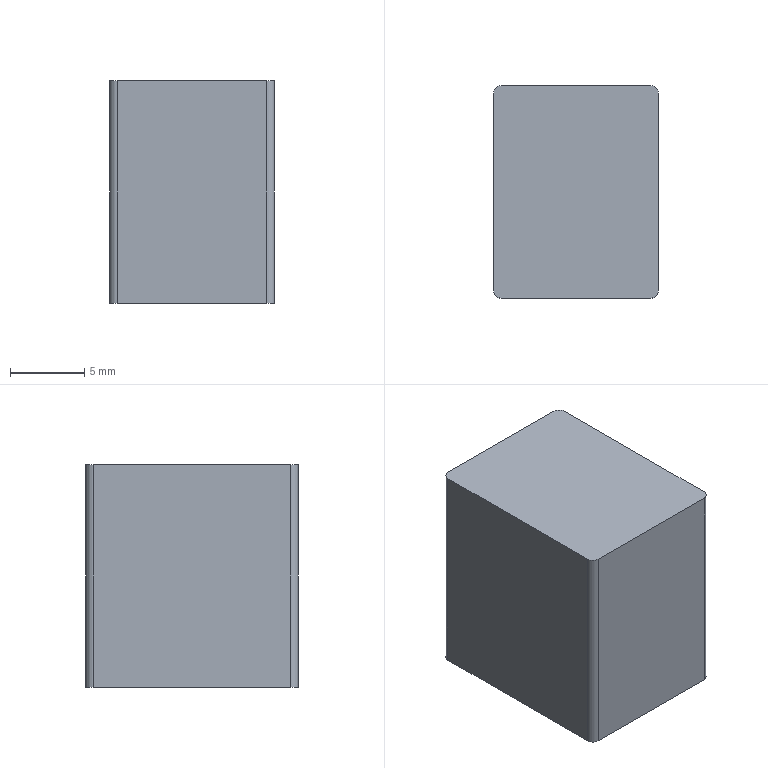Part | NX | features BREP 1 | 1 solid | 10 faces | box 11.115 x 14.326 x 15 mm | volume 2385 mm3 | plane 6 | cylinder 4 | commonest cylinder face diameters 1 x4
STEP:
#1=CARTESIAN_POINT('',(-5.058,7.163,-25.6));
#2=VERTEX_POINT('',#1);
#3=CARTESIAN_POINT('',(-5.558,6.663,-25.6));
#4=VERTEX_POINT('',#3);
#5=CARTESIAN_POINT('',(-5.058,6.663,-25.6));
#6=DIRECTION('',(0.,0.,1.));
#7=DIRECTION('',(1.,0.,0.));
#8=AXIS2_PLACEMENT_3D('',#5,#6,#7);
#9=CIRCLE('',#8,0.5);
#10=EDGE_CURVE('',#2,#4,#9,.T.);
#11=ORIENTED_EDGE('',*,*,#10,.F.);
#12=CARTESIAN_POINT('',(-5.058,7.163,-40.6));
#13=VERTEX_POINT('',#12);
#14=CARTESIAN_POINT('',(-5.058,7.163,-40.6));
#15=DIRECTION('',(0.,0.,1.));
#16=VECTOR('',#15,1000.);
#17=LINE('',#14,#16);
#18=EDGE_CURVE('',#13,#2,#17,.T.);
#19=ORIENTED_EDGE('',*,*,#18,.F.);
#20=CARTESIAN_POINT('',(-5.558,6.663,-40.6));
#21=VERTEX_POINT('',#20);
#22=CARTESIAN_POINT('',(-5.058,6.663,-40.6));
#23=DIRECTION('',(0.,0.,1.));
#24=DIRECTION('',(1.,0.,0.));
#25=AXIS2_PLACEMENT_3D('',#22,#23,#24);
#26=CIRCLE('',#25,0.5);
#27=EDGE_CURVE('',#13,#21,#26,.T.);
#28=ORIENTED_EDGE('',*,*,#27,.T.);
#29=CARTESIAN_POINT('',(-5.558,6.663,-40.6));
#30=DIRECTION('',(0.,0.,1.));
#31=VECTOR('',#30,1000.);
#32=LINE('',#29,#31);
#33=EDGE_CURVE('',#21,#4,#32,.T.);
#34=ORIENTED_EDGE('',*,*,#33,.T.);
#35=EDGE_LOOP('',(#11,#19,#28,#34));
#36=FACE_BOUND('',#35,.T.);
#37=CARTESIAN_POINT('',(-5.058,6.663,-40.6));
#38=DIRECTION('',(0.,0.,1.));
#39=DIRECTION('',(-1.,0.,0.));
#40=AXIS2_PLACEMENT_3D('',#37,#38,#39);
#41=CYLINDRICAL_SURFACE('',#40,0.5);
#42=ADVANCED_FACE('',(#36),#41,.T.);
#43=CARTESIAN_POINT('',(-5.558,-6.663,-25.6));
#44=VERTEX_POINT('',#43);
#45=CARTESIAN_POINT('',(-5.558,-6.663,-25.6));
#46=DIRECTION('',(0.,1.,0.));
#47=VECTOR('',#46,1000.);
#48=LINE('',#45,#47);
#49=EDGE_CURVE('',#44,#4,#48,.T.);
#50=ORIENTED_EDGE('',*,*,#49,.T.);
#51=ORIENTED_EDGE('',*,*,#33,.F.);
#52=CARTESIAN_POINT('',(-5.558,-6.663,-40.6));
#53=VERTEX_POINT('',#52);
#54=CARTESIAN_POINT('',(-5.558,-6.663,-40.6));
#55=DIRECTION('',(0.,1.,0.));
#56=VECTOR('',#55,1000.);
#57=LINE('',#54,#56);
#58=EDGE_CURVE('',#53,#21,#57,.T.);
#59=ORIENTED_EDGE('',*,*,#58,.F.);
#60=CARTESIAN_POINT('',(-5.558,-6.663,-40.6));
#61=DIRECTION('',(0.,0.,1.));
#62=VECTOR('',#61,1000.);
#63=LINE('',#60,#62);
#64=EDGE_CURVE('',#53,#44,#63,.T.);
#65=ORIENTED_EDGE('',*,*,#64,.T.);
#66=EDGE_LOOP('',(#50,#51,#59,#65));
#67=FACE_BOUND('',#66,.T.);
#68=CARTESIAN_POINT('',(-5.558,-6.663,-40.6));
#69=DIRECTION('',(1.,0.,0.));
#70=DIRECTION('',(0.,0.,1.));
#71=AXIS2_PLACEMENT_3D('',#68,#69,#70);
#72=PLANE('',#71);
#73=ADVANCED_FACE('',(#67),#72,.F.);
#74=CARTESIAN_POINT('',(-5.058,-7.163,-25.6));
#75=VERTEX_POINT('',#74);
#76=CARTESIAN_POINT('',(-5.058,-6.663,-25.6));
#77=DIRECTION('',(0.,0.,1.));
#78=DIRECTION('',(1.,0.,0.));
#79=AXIS2_PLACEMENT_3D('',#76,#77,#78);
#80=CIRCLE('',#79,0.5);
#81=EDGE_CURVE('',#44,#75,#80,.T.);
#82=ORIENTED_EDGE('',*,*,#81,.F.);
#83=ORIENTED_EDGE('',*,*,#64,.F.);
#84=CARTESIAN_POINT('',(-5.058,-7.163,-40.6));
#85=VERTEX_POINT('',#84);
#86=CARTESIAN_POINT('',(-5.058,-6.663,-40.6));
#87=DIRECTION('',(0.,0.,1.));
#88=DIRECTION('',(1.,0.,0.));
#89=AXIS2_PLACEMENT_3D('',#86,#87,#88);
#90=CIRCLE('',#89,0.5);
#91=EDGE_CURVE('',#53,#85,#90,.T.);
#92=ORIENTED_EDGE('',*,*,#91,.T.);
#93=CARTESIAN_POINT('',(-5.058,-7.163,-40.6));
#94=DIRECTION('',(0.,0.,1.));
#95=VECTOR('',#94,1000.);
#96=LINE('',#93,#95);
#97=EDGE_CURVE('',#85,#75,#96,.T.);
#98=ORIENTED_EDGE('',*,*,#97,.T.);
#99=EDGE_LOOP('',(#82,#83,#92,#98));
#100=FACE_BOUND('',#99,.T.);
#101=CARTESIAN_POINT('',(-5.058,-6.663,-40.6));
#102=DIRECTION('',(0.,0.,1.));
#103=DIRECTION('',(-1.,0.,0.));
#104=AXIS2_PLACEMENT_3D('',#101,#102,#103);
#105=CYLINDRICAL_SURFACE('',#104,0.5);
#106=ADVANCED_FACE('',(#100),#105,.T.);
#107=CARTESIAN_POINT('',(5.058,-7.163,-25.6));
#108=VERTEX_POINT('',#107);
#109=CARTESIAN_POINT('',(5.058,-7.163,-25.6));
#110=DIRECTION('',(-1.,0.,0.));
#111=VECTOR('',#110,1000.);
#112=LINE('',#109,#111);
#113=EDGE_CURVE('',#108,#75,#112,.T.);
#114=ORIENTED_EDGE('',*,*,#113,.T.);
#115=ORIENTED_EDGE('',*,*,#97,.F.);
#116=CARTESIAN_POINT('',(5.058,-7.163,-40.6));
#117=VERTEX_POINT('',#116);
#118=CARTESIAN_POINT('',(5.058,-7.163,-40.6));
#119=DIRECTION('',(-1.,0.,0.));
#120=VECTOR('',#119,1000.);
#121=LINE('',#118,#120);
#122=EDGE_CURVE('',#117,#85,#121,.T.);
#123=ORIENTED_EDGE('',*,*,#122,.F.);
#124=CARTESIAN_POINT('',(5.058,-7.163,-40.6));
#125=DIRECTION('',(0.,0.,1.));
#126=VECTOR('',#125,1000.);
#127=LINE('',#124,#126);
#128=EDGE_CURVE('',#117,#108,#127,.T.);
#129=ORIENTED_EDGE('',*,*,#128,.T.);
#130=EDGE_LOOP('',(#114,#115,#123,#129));
#131=FACE_BOUND('',#130,.T.);
#132=CARTESIAN_POINT('',(5.058,-7.163,-40.6));
#133=DIRECTION('',(0.,1.,0.));
#134=DIRECTION('',(0.,0.,-1.));
#135=AXIS2_PLACEMENT_3D('',#132,#133,#134);
#136=PLANE('',#135);
#137=ADVANCED_FACE('',(#131),#136,.F.);
#138=CARTESIAN_POINT('',(5.558,-6.663,-25.6));
#139=VERTEX_POINT('',#138);
#140=CARTESIAN_POINT('',(5.058,-6.663,-25.6));
#141=DIRECTION('',(0.,0.,1.));
#142=DIRECTION('',(1.,0.,0.));
#143=AXIS2_PLACEMENT_3D('',#140,#141,#142);
#144=CIRCLE('',#143,0.5);
#145=EDGE_CURVE('',#108,#139,#144,.T.);
#146=ORIENTED_EDGE('',*,*,#145,.F.);
#147=ORIENTED_EDGE('',*,*,#128,.F.);
#148=CARTESIAN_POINT('',(5.558,-6.663,-40.6));
#149=VERTEX_POINT('',#148);
#150=CARTESIAN_POINT('',(5.058,-6.663,-40.6));
#151=DIRECTION('',(0.,0.,1.));
#152=DIRECTION('',(1.,0.,0.));
#153=AXIS2_PLACEMENT_3D('',#150,#151,#152);
#154=CIRCLE('',#153,0.5);
#155=EDGE_CURVE('',#117,#149,#154,.T.);
#156=ORIENTED_EDGE('',*,*,#155,.T.);
#157=CARTESIAN_POINT('',(5.558,-6.663,-40.6));
#158=DIRECTION('',(0.,0.,1.));
#159=VECTOR('',#158,1000.);
#160=LINE('',#157,#159);
#161=EDGE_CURVE('',#149,#139,#160,.T.);
#162=ORIENTED_EDGE('',*,*,#161,.T.);
#163=EDGE_LOOP('',(#146,#147,#156,#162));
#164=FACE_BOUND('',#163,.T.);
#165=CARTESIAN_POINT('',(5.058,-6.663,-40.6));
#166=DIRECTION('',(0.,0.,1.));
#167=DIRECTION('',(-1.,0.,0.));
#168=AXIS2_PLACEMENT_3D('',#165,#166,#167);
#169=CYLINDRICAL_SURFACE('',#168,0.5);
#170=ADVANCED_FACE('',(#164),#169,.T.);
#171=CARTESIAN_POINT('',(5.558,6.663,-25.6));
#172=VERTEX_POINT('',#171);
#173=CARTESIAN_POINT('',(5.558,6.663,-25.6));
#174=DIRECTION('',(0.,-1.,0.));
#175=VECTOR('',#174,1000.);
#176=LINE('',#173,#175);
#177=EDGE_CURVE('',#172,#139,#176,.T.);
#178=ORIENTED_EDGE('',*,*,#177,.T.);
#179=ORIENTED_EDGE('',*,*,#161,.F.);
#180=CARTESIAN_POINT('',(5.558,6.663,-40.6));
#181=VERTEX_POINT('',#180);
#182=CARTESIAN_POINT('',(5.558,6.663,-40.6));
#183=DIRECTION('',(0.,-1.,0.));
#184=VECTOR('',#183,1000.);
#185=LINE('',#182,#184);
#186=EDGE_CURVE('',#181,#149,#185,.T.);
#187=ORIENTED_EDGE('',*,*,#186,.F.);
#188=CARTESIAN_POINT('',(5.558,6.663,-40.6));
#189=DIRECTION('',(0.,0.,1.));
#190=VECTOR('',#189,1000.);
#191=LINE('',#188,#190);
#192=EDGE_CURVE('',#181,#172,#191,.T.);
#193=ORIENTED_EDGE('',*,*,#192,.T.);
#194=EDGE_LOOP('',(#178,#179,#187,#193));
#195=FACE_BOUND('',#194,.T.);
#196=CARTESIAN_POINT('',(5.558,6.663,-40.6));
#197=DIRECTION('',(-1.,0.,0.));
#198=DIRECTION('',(0.,0.,-1.));
#199=AXIS2_PLACEMENT_3D('',#196,#197,#198);
#200=PLANE('',#199);
#201=ADVANCED_FACE('',(#195),#200,.F.);
#202=CARTESIAN_POINT('',(5.058,7.163,-25.6));
#203=VERTEX_POINT('',#202);
#204=CARTESIAN_POINT('',(5.058,6.663,-25.6));
#205=DIRECTION('',(0.,0.,1.));
#206=DIRECTION('',(1.,0.,0.));
#207=AXIS2_PLACEMENT_3D('',#204,#205,#206);
#208=CIRCLE('',#207,0.5);
#209=EDGE_CURVE('',#172,#203,#208,.T.);
#210=ORIENTED_EDGE('',*,*,#209,.F.);
#211=ORIENTED_EDGE('',*,*,#192,.F.);
#212=CARTESIAN_POINT('',(5.058,7.163,-40.6));
#213=VERTEX_POINT('',#212);
#214=CARTESIAN_POINT('',(5.058,6.663,-40.6));
#215=DIRECTION('',(0.,0.,1.));
#216=DIRECTION('',(1.,0.,0.));
#217=AXIS2_PLACEMENT_3D('',#214,#215,#216);
#218=CIRCLE('',#217,0.5);
#219=EDGE_CURVE('',#181,#213,#218,.T.);
#220=ORIENTED_EDGE('',*,*,#219,.T.);
#221=CARTESIAN_POINT('',(5.058,7.163,-40.6));
#222=DIRECTION('',(0.,0.,1.));
#223=VECTOR('',#222,1000.);
#224=LINE('',#221,#223);
#225=EDGE_CURVE('',#213,#203,#224,.T.);
#226=ORIENTED_EDGE('',*,*,#225,.T.);
#227=EDGE_LOOP('',(#210,#211,#220,#226));
#228=FACE_BOUND('',#227,.T.);
#229=CARTESIAN_POINT('',(5.058,6.663,-40.6));
#230=DIRECTION('',(0.,0.,1.));
#231=DIRECTION('',(-1.,0.,0.));
#232=AXIS2_PLACEMENT_3D('',#229,#230,#231);
#233=CYLINDRICAL_SURFACE('',#232,0.5);
#234=ADVANCED_FACE('',(#228),#233,.T.);
#235=CARTESIAN_POINT('',(-5.058,7.163,-25.6));
#236=DIRECTION('',(1.,0.,0.));
#237=VECTOR('',#236,1000.);
#238=LINE('',#235,#237);
#239=EDGE_CURVE('',#2,#203,#238,.T.);
#240=ORIENTED_EDGE('',*,*,#239,.T.);
#241=ORIENTED_EDGE('',*,*,#225,.F.);
#242=CARTESIAN_POINT('',(-5.058,7.163,-40.6));
#243=DIRECTION('',(1.,0.,0.));
#244=VECTOR('',#243,1000.);
#245=LINE('',#242,#244);
#246=EDGE_CURVE('',#13,#213,#245,.T.);
#247=ORIENTED_EDGE('',*,*,#246,.F.);
#248=ORIENTED_EDGE('',*,*,#18,.T.);
#249=EDGE_LOOP('',(#240,#241,#247,#248));
#250=FACE_BOUND('',#249,.T.);
#251=CARTESIAN_POINT('',(-5.058,7.163,-40.6));
#252=DIRECTION('',(0.,-1.,0.));
#253=DIRECTION('',(0.,0.,1.));
#254=AXIS2_PLACEMENT_3D('',#251,#252,#253);
#255=PLANE('',#254);
#256=ADVANCED_FACE('',(#250),#255,.F.);
#257=ORIENTED_EDGE('',*,*,#27,.F.);
#258=ORIENTED_EDGE('',*,*,#246,.T.);
#259=ORIENTED_EDGE('',*,*,#219,.F.);
#260=ORIENTED_EDGE('',*,*,#186,.T.);
#261=ORIENTED_EDGE('',*,*,#155,.F.);
#262=ORIENTED_EDGE('',*,*,#122,.T.);
#263=ORIENTED_EDGE('',*,*,#91,.F.);
#264=ORIENTED_EDGE('',*,*,#58,.T.);
#265=EDGE_LOOP('',(#257,#258,#259,#260,#261,#262,#263,#264));
#266=FACE_BOUND('',#265,.T.);
#267=CARTESIAN_POINT('',(-5.058,6.663,-40.6));
#268=DIRECTION('',(0.,0.,1.));
#269=DIRECTION('',(-1.,0.,0.));
#270=AXIS2_PLACEMENT_3D('',#267,#268,#269);
#271=PLANE('',#270);
#272=ADVANCED_FACE('',(#266),#271,.F.);
#273=ORIENTED_EDGE('',*,*,#10,.T.);
#274=ORIENTED_EDGE('',*,*,#49,.F.);
#275=ORIENTED_EDGE('',*,*,#81,.T.);
#276=ORIENTED_EDGE('',*,*,#113,.F.);
#277=ORIENTED_EDGE('',*,*,#145,.T.);
#278=ORIENTED_EDGE('',*,*,#177,.F.);
#279=ORIENTED_EDGE('',*,*,#209,.T.);
#280=ORIENTED_EDGE('',*,*,#239,.F.);
#281=EDGE_LOOP('',(#273,#274,#275,#276,#277,#278,#279,#280));
#282=FACE_BOUND('',#281,.T.);
#283=CARTESIAN_POINT('',(-5.058,6.663,-25.6));
#284=DIRECTION('',(0.,0.,1.));
#285=DIRECTION('',(-1.,0.,0.));
#286=AXIS2_PLACEMENT_3D('',#283,#284,#285);
#287=PLANE('',#286);
#288=ADVANCED_FACE('',(#282),#287,.T.);
#289=CLOSED_SHELL('',(#42,#73,#106,#137,#170,#201,#234,#256,#272,#288));
#290=MANIFOLD_SOLID_BREP('',#289);
#291=(LENGTH_UNIT()NAMED_UNIT(*)SI_UNIT(.MILLI.,.METRE.));
#292=UNCERTAINTY_MEASURE_WITH_UNIT(LENGTH_MEASURE(0.00001),#291,'','');
#293=(NAMED_UNIT(*)PLANE_ANGLE_UNIT()SI_UNIT($,.RADIAN.));
#294=(NAMED_UNIT(*)SI_UNIT($,.STERADIAN.)SOLID_ANGLE_UNIT());
#295=(GEOMETRIC_REPRESENTATION_CONTEXT(3)GLOBAL_UNCERTAINTY_ASSIGNED_CONTEXT((#292))GLOBAL_UNIT_ASSIGNED_CONTEXT((#291,#293,#294))REPRESENTATION_CONTEXT('',''));
#296=ADVANCED_BREP_SHAPE_REPRESENTATION('',(#290),#295);